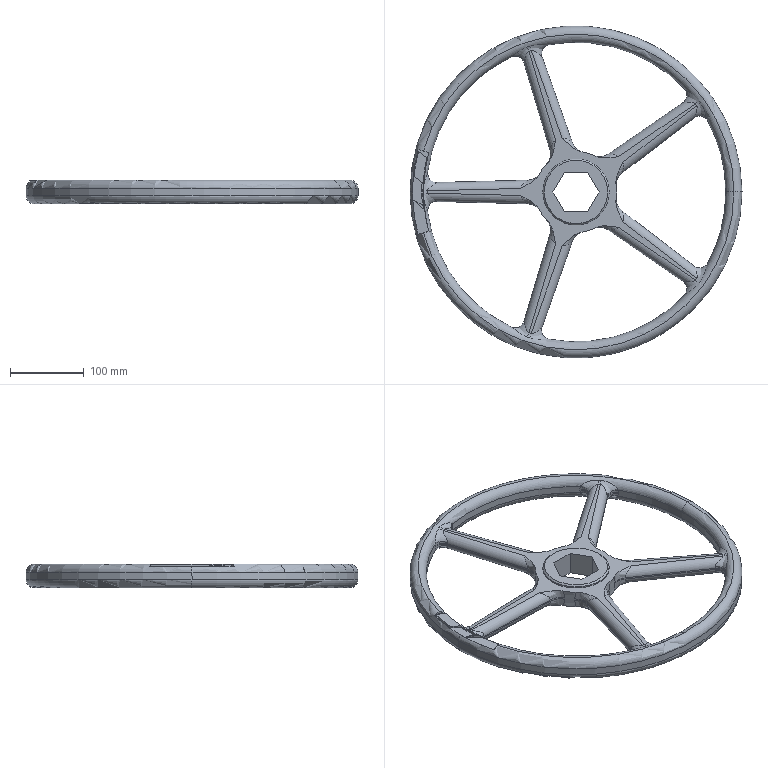Part | SolidWorks | features ICE 5, Fillet 4, MoveFace 2, Blend 1, Chamfer 1, CirPattern 1, CombineBodies 1, Extrusion 1 | 1 solid | 181 faces | box 450 x 450 x 32 mm | volume 1456731 mm3 | cylinder 71 | spline 60 | plane 28 | torus 18 | cone 4 | commonest cylinder face diameters 22 x20 24 x14 40 x12 110 x5 406 x5 90 x4